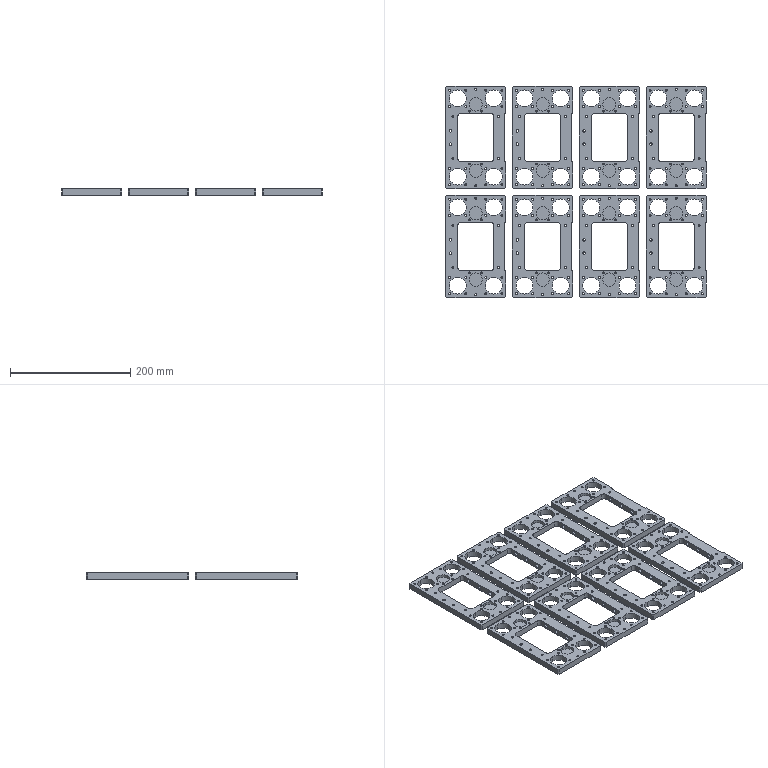NC program | NX | posted with a generic post | part box 433 x 351 x 10 mm
Lines 530 to 1335 of 15742:
(ZLEVEL_PROFILE , TOOL : D10)
N1046 T15 M6
N1048 G54
N1050 G17 G0 G90 X-221.6 Y-137.058 B0. C0. S9500 M3
N1052 G43 Z30. H15
N1054 Z1.5
N1056 G94 G1 Y-90.5 Z-0.94 F1000.
N1058 Y-7.5 F3000.
N1060 G2 X-220.106 Y-3.894 R5.1
N1062 G1 X-218.106 Y-1.894
N1064 G2 X-214.5 Y-0.4 R5.1
N1066 G1 X-118.5
N1068 G2 X-114.894 Y-1.894 R5.1
N1070 G1 X-112.894 Y-3.894
N1072 G2 X-111.4 Y-7.5 R5.1
N1074 G1 Y-50.5
N1076 G2 X-113.4 Y-54.55 R5.1
N1078 G1 Y-126.45
N1080 G2 X-111.4 Y-130.5 R5.1
N1082 G1 Y-173.5
N1084 G2 X-112.894 Y-177.106 R5.1
N1086 G1 X-114.894 Y-179.106
N1088 G2 X-118.5 Y-180.6 R5.1
N1090 G1 X-214.5
N1092 G2 X-218.106 Y-179.106 R5.1
N1094 G1 X-220.106 Y-177.106
N1096 G2 X-221.6 Y-173.5 R5.1
N1098 G1 Y-90.5
N1100 Y-7.5 Z-1.077
N1102 X-221.575 Y-7. Z-1.078
N1104 X-221.502 Y-6.505 Z-1.079
N1106 X-221.38 Y-6.02 Z-1.08
N1108 X-221.212 Y-5.548 Z-1.081
N1110 X-220.998 Y-5.096
N1112 X-220.74 Y-4.667 Z-1.082
N1114 X-220.442 Y-4.265 Z-1.083
N1116 X-220.106 Y-3.894 Z-1.084
N1118 X-218.106 Y-1.894 Z-1.089
N1120 X-217.735 Y-1.558
N1122 X-217.333 Y-1.26 Z-1.09
N1124 X-216.904 Y-1.002 Z-1.091
N1126 X-216.452 Y-0.788 Z-1.092
N1128 X-215.98 Y-0.62 Z-1.093
N1130 X-215.495 Y-0.498
N1132 X-215. Y-0.425 Z-1.094
N1134 X-214.5 Y-0.4 Z-1.095
N1136 X-118.5 Z-1.254
N1138 X-118. Y-0.425 Z-1.255
N1140 X-117.505 Y-0.498
N1142 X-117.02 Y-0.62 Z-1.256
N1144 X-116.548 Y-0.788 Z-1.257
N1146 X-116.096 Y-1.002 Z-1.258
N1148 X-115.667 Y-1.26 Z-1.259
N1150 X-115.265 Y-1.558 Z-1.26
N1152 X-114.894 Y-1.894
N1154 X-112.894 Y-3.894 Z-1.265
N1156 X-112.558 Y-4.265 Z-1.266
N1158 X-112.26 Y-4.667 Z-1.267
N1160 X-112.002 Y-5.096 Z-1.268
N1162 X-111.788 Y-5.548
N1164 X-111.62 Y-6.02 Z-1.269
N1166 X-111.498 Y-6.505 Z-1.27
N1168 X-111.425 Y-7. Z-1.271
N1170 X-111.4 Y-7.5 Z-1.272
N1172 Y-50.5 Z-1.343
N1174 X-111.421 Y-50.967 Z-1.344
N1176 X-111.486 Y-51.431
N1178 X-111.592 Y-51.886 Z-1.345
N1180 X-111.74 Y-52.33 Z-1.346
N1182 X-111.927 Y-52.758 Z-1.347
N1184 X-112.153 Y-53.168
N1186 X-112.416 Y-53.555 Z-1.348
N1188 X-112.713 Y-53.916 Z-1.349
N1190 X-113.038 Y-54.245 Z-1.35
N1192 X-113.4 Y-54.55 Z-1.351
N1194 Y-126.45 Z-1.469
N1196 X-113.034 Y-126.758 Z-1.47
N1198 X-112.713 Y-127.084 Z-1.471
N1200 X-112.416 Y-127.445 Z-1.472
N1202 X-112.153 Y-127.832 Z-1.473
N1204 X-111.927 Y-128.242
N1206 X-111.74 Y-128.67 Z-1.474
N1208 X-111.592 Y-129.114 Z-1.475
N1210 X-111.486 Y-129.569 Z-1.476
N1212 X-111.421 Y-130.033
N1214 X-111.4 Y-130.5 Z-1.477
N1216 Y-173.5 Z-1.548
N1218 X-111.425 Y-174. Z-1.549
N1220 X-111.498 Y-174.495 Z-1.55
N1222 X-111.62 Y-174.98 Z-1.551
N1224 X-111.788 Y-175.452 Z-1.552
N1226 X-112.002 Y-175.904
N1228 X-112.26 Y-176.333 Z-1.553
N1230 X-112.558 Y-176.735 Z-1.554
N1232 X-112.894 Y-177.106 Z-1.555
N1234 X-114.894 Y-179.106 Z-1.56
N1236 X-115.265 Y-179.442
N1238 X-115.667 Y-179.74 Z-1.561
N1240 X-116.096 Y-179.998 Z-1.562
N1242 X-116.548 Y-180.212 Z-1.563
N1244 X-117.02 Y-180.38 Z-1.564
N1246 X-117.505 Y-180.502 Z-1.565
N1248 X-118. Y-180.575
N1250 X-118.5 Y-180.6 Z-1.566
N1252 X-214.5 Z-1.725
N1254 X-215. Y-180.575 Z-1.726
N1256 X-215.495 Y-180.502 Z-1.727
N1258 X-215.98 Y-180.38
N1260 X-216.452 Y-180.212 Z-1.728
N1262 X-216.904 Y-179.998 Z-1.729
N1264 X-217.333 Y-179.74 Z-1.73
N1266 X-217.735 Y-179.442 Z-1.731
N1268 X-218.106 Y-179.106
N1270 X-220.106 Y-177.106 Z-1.736
N1272 X-220.442 Y-176.735 Z-1.737
N1274 X-220.74 Y-176.333 Z-1.738
N1276 X-220.998 Y-175.904 Z-1.739
N1278 X-221.212 Y-175.452
N1280 X-221.38 Y-174.98 Z-1.74
N1282 X-221.502 Y-174.495 Z-1.741
N1284 X-221.575 Y-174. Z-1.742
N1286 X-221.6 Y-173.5 Z-1.743
N1288 Y-90.5 Z-1.88
N1290 Y-7.5 Z-2.017
N1292 X-221.575 Y-7. Z-2.018
N1294 X-221.502 Y-6.505 Z-2.019
N1296 X-221.38 Y-6.02 Z-2.02
N1298 X-221.212 Y-5.548 Z-2.021
N1300 X-220.998 Y-5.096
N1302 X-220.74 Y-4.667 Z-2.022
N1304 X-220.442 Y-4.265 Z-2.023
N1306 X-220.106 Y-3.894 Z-2.024
N1308 X-218.106 Y-1.894 Z-2.029
N1310 X-217.735 Y-1.558
N1312 X-217.333 Y-1.26 Z-2.03
N1314 X-216.904 Y-1.002 Z-2.031
N1316 X-216.452 Y-0.788 Z-2.032
N1318 X-215.98 Y-0.62 Z-2.033
N1320 X-215.495 Y-0.498
N1322 X-215. Y-0.425 Z-2.034
N1324 X-214.5 Y-0.4 Z-2.035
N1326 X-118.5 Z-2.194
N1328 X-118. Y-0.425 Z-2.195
N1330 X-117.505 Y-0.498
N1332 X-117.02 Y-0.62 Z-2.196
N1334 X-116.548 Y-0.788 Z-2.197
N1336 X-116.096 Y-1.002 Z-2.198
N1338 X-115.667 Y-1.26 Z-2.199
N1340 X-115.265 Y-1.558 Z-2.2
N1342 X-114.894 Y-1.894
N1344 X-112.894 Y-3.894 Z-2.205
N1346 X-112.558 Y-4.265 Z-2.206
N1348 X-112.26 Y-4.667 Z-2.207
N1350 X-112.002 Y-5.096 Z-2.208
N1352 X-111.788 Y-5.548
N1354 X-111.62 Y-6.02 Z-2.209
N1356 X-111.498 Y-6.505 Z-2.21
N1358 X-111.425 Y-7. Z-2.211
N1360 X-111.4 Y-7.5 Z-2.212
N1362 Y-50.5 Z-2.283
N1364 X-111.421 Y-50.967 Z-2.284
N1366 X-111.486 Y-51.431
N1368 X-111.592 Y-51.886 Z-2.285
N1370 X-111.74 Y-52.33 Z-2.286
N1372 X-111.927 Y-52.758 Z-2.287
N1374 X-112.153 Y-53.168
N1376 X-112.416 Y-53.555 Z-2.288
N1378 X-112.713 Y-53.916 Z-2.289
N1380 X-113.038 Y-54.245 Z-2.29
N1382 X-113.4 Y-54.55 Z-2.291
N1384 Y-126.45 Z-2.409
N1386 X-113.034 Y-126.758 Z-2.41
N1388 X-112.713 Y-127.084 Z-2.411
N1390 X-112.416 Y-127.445 Z-2.412
N1392 X-112.153 Y-127.832 Z-2.413
N1394 X-111.927 Y-128.242
N1396 X-111.74 Y-128.67 Z-2.414
N1398 X-111.592 Y-129.114 Z-2.415
N1400 X-111.486 Y-129.569 Z-2.416
N1402 X-111.421 Y-130.033
N1404 X-111.4 Y-130.5 Z-2.417
N1406 Y-173.5 Z-2.488
N1408 X-111.425 Y-174. Z-2.489
N1410 X-111.498 Y-174.495 Z-2.49
N1412 X-111.62 Y-174.98 Z-2.491
N1414 X-111.788 Y-175.452 Z-2.492
N1416 X-112.002 Y-175.904
N1418 X-112.26 Y-176.333 Z-2.493
N1420 X-112.558 Y-176.735 Z-2.494
N1422 X-112.894 Y-177.106 Z-2.495
N1424 X-114.894 Y-179.106 Z-2.5
N1426 X-115.265 Y-179.442
N1428 X-115.667 Y-179.74 Z-2.501
N1430 X-116.096 Y-179.998 Z-2.502
N1432 X-116.548 Y-180.212 Z-2.503
N1434 X-117.02 Y-180.38 Z-2.504
N1436 X-117.505 Y-180.502 Z-2.505
N1438 X-118. Y-180.575
N1440 X-118.5 Y-180.6 Z-2.506
N1442 X-214.5 Z-2.665
N1444 X-215. Y-180.575 Z-2.666
N1446 X-215.495 Y-180.502 Z-2.667
N1448 X-215.98 Y-180.38
N1450 X-216.452 Y-180.212 Z-2.668
N1452 X-216.904 Y-179.998 Z-2.669
N1454 X-217.333 Y-179.74 Z-2.67
N1456 X-217.735 Y-179.442 Z-2.671
N1458 X-218.106 Y-179.106
N1460 X-220.106 Y-177.106 Z-2.676
N1462 X-220.442 Y-176.735 Z-2.677
N1464 X-220.74 Y-176.333 Z-2.678
N1466 X-220.998 Y-175.904 Z-2.679
N1468 X-221.212 Y-175.452
N1470 X-221.38 Y-174.98 Z-2.68
N1472 X-221.502 Y-174.495 Z-2.681
N1474 X-221.575 Y-174. Z-2.682
N1476 X-221.6 Y-173.5 Z-2.683
N1478 Y-90.5 Z-2.82
N1480 Y-7.5 Z-2.957
N1482 X-221.575 Y-7. Z-2.958
N1484 X-221.502 Y-6.505 Z-2.959
N1486 X-221.38 Y-6.02 Z-2.96
N1488 X-221.212 Y-5.548 Z-2.961
N1490 X-220.998 Y-5.096
N1492 X-220.74 Y-4.667 Z-2.962
N1494 X-220.442 Y-4.265 Z-2.963
N1496 X-220.106 Y-3.894 Z-2.964
N1498 X-218.106 Y-1.894 Z-2.969
N1500 X-217.735 Y-1.558
N1502 X-217.333 Y-1.26 Z-2.97
N1504 X-216.904 Y-1.002 Z-2.971
N1506 X-216.452 Y-0.788 Z-2.972
N1508 X-215.98 Y-0.62 Z-2.973
N1510 X-215.495 Y-0.498
N1512 X-215. Y-0.425 Z-2.974
N1514 X-214.5 Y-0.4 Z-2.975
N1516 X-118.5 Z-3.134
N1518 X-118. Y-0.425 Z-3.135
N1520 X-117.505 Y-0.498
N1522 X-117.02 Y-0.62 Z-3.136
N1524 X-116.548 Y-0.788 Z-3.137
N1526 X-116.096 Y-1.002 Z-3.138
N1528 X-115.667 Y-1.26 Z-3.139
N1530 X-115.265 Y-1.558 Z-3.14
N1532 X-114.894 Y-1.894
N1534 X-112.894 Y-3.894 Z-3.145
N1536 X-112.558 Y-4.265 Z-3.146
N1538 X-112.26 Y-4.667 Z-3.147
N1540 X-112.002 Y-5.096 Z-3.148
N1542 X-111.788 Y-5.548
N1544 X-111.62 Y-6.02 Z-3.149
N1546 X-111.498 Y-6.505 Z-3.15
N1548 X-111.425 Y-7. Z-3.151
N1550 X-111.4 Y-7.5 Z-3.152
N1552 Y-50.5 Z-3.223
N1554 X-111.421 Y-50.967 Z-3.224
N1556 X-111.486 Y-51.431
N1558 X-111.592 Y-51.886 Z-3.225
N1560 X-111.74 Y-52.33 Z-3.226
N1562 X-111.927 Y-52.758 Z-3.227
N1564 X-112.153 Y-53.168
N1566 X-112.416 Y-53.555 Z-3.228
N1568 X-112.713 Y-53.916 Z-3.229
N1570 X-113.038 Y-54.245 Z-3.23
N1572 X-113.4 Y-54.55 Z-3.231
N1574 Y-126.45 Z-3.349
N1576 X-113.034 Y-126.758 Z-3.35
N1578 X-112.713 Y-127.084 Z-3.351
N1580 X-112.416 Y-127.445 Z-3.352
N1582 X-112.153 Y-127.832 Z-3.353
N1584 X-111.927 Y-128.242
N1586 X-111.74 Y-128.67 Z-3.354
N1588 X-111.592 Y-129.114 Z-3.355
N1590 X-111.486 Y-129.569 Z-3.356
N1592 X-111.421 Y-130.033
N1594 X-111.4 Y-130.5 Z-3.357
N1596 Y-173.5 Z-3.428
N1598 X-111.425 Y-174. Z-3.429
N1600 X-111.498 Y-174.495 Z-3.43
N1602 X-111.62 Y-174.98 Z-3.431
N1604 X-111.788 Y-175.452 Z-3.432
N1606 X-112.002 Y-175.904
N1608 X-112.26 Y-176.333 Z-3.433
N1610 X-112.558 Y-176.735 Z-3.434
N1612 X-112.894 Y-177.106 Z-3.435
N1614 X-114.894 Y-179.106 Z-3.44
N1616 X-115.265 Y-179.442
N1618 X-115.667 Y-179.74 Z-3.441
N1620 X-116.096 Y-179.998 Z-3.442
N1622 X-116.548 Y-180.212 Z-3.443
N1624 X-117.02 Y-180.38 Z-3.444
N1626 X-117.505 Y-180.502 Z-3.445
N1628 X-118. Y-180.575
N1630 X-118.5 Y-180.6 Z-3.446
N1632 X-214.5 Z-3.605
N1634 X-215. Y-180.575 Z-3.606
N1636 X-215.495 Y-180.502 Z-3.607
N1638 X-215.98 Y-180.38
N1640 X-216.452 Y-180.212 Z-3.608
N1642 X-216.904 Y-179.998 Z-3.609
N1644 X-217.333 Y-179.74 Z-3.61
N1646 X-217.735 Y-179.442 Z-3.611
N1648 X-218.106 Y-179.106
N1650 X-220.106 Y-177.106 Z-3.616
N1652 X-220.442 Y-176.735 Z-3.617
N1654 X-220.74 Y-176.333 Z-3.618
N1656 X-220.998 Y-175.904 Z-3.619
N1658 X-221.212 Y-175.452
N1660 X-221.38 Y-174.98 Z-3.62
N1662 X-221.502 Y-174.495 Z-3.621
N1664 X-221.575 Y-174. Z-3.622
N1666 X-221.6 Y-173.5 Z-3.623
N1668 Y-90.5 Z-3.76
N1670 Y-7.5 Z-3.897
N1672 X-221.575 Y-7. Z-3.898
N1674 X-221.502 Y-6.505 Z-3.899
N1676 X-221.38 Y-6.02 Z-3.9
N1678 X-221.212 Y-5.548 Z-3.901
N1680 X-220.998 Y-5.096
N1682 X-220.74 Y-4.667 Z-3.902
N1684 X-220.442 Y-4.265 Z-3.903
N1686 X-220.106 Y-3.894 Z-3.904
N1688 X-218.106 Y-1.894 Z-3.909
N1690 X-217.735 Y-1.558
N1692 X-217.333 Y-1.26 Z-3.91
N1694 X-216.904 Y-1.002 Z-3.911
N1696 X-216.452 Y-0.788 Z-3.912
N1698 X-215.98 Y-0.62 Z-3.913
N1700 X-215.495 Y-0.498
N1702 X-215. Y-0.425 Z-3.914
N1704 X-214.5 Y-0.4 Z-3.915
N1706 X-118.5 Z-4.074
N1708 X-118. Y-0.425 Z-4.075
N1710 X-117.505 Y-0.498
N1712 X-117.02 Y-0.62 Z-4.076
N1714 X-116.548 Y-0.788 Z-4.077
N1716 X-116.096 Y-1.002 Z-4.078
N1718 X-115.667 Y-1.26 Z-4.079
N1720 X-115.265 Y-1.558 Z-4.08
N1722 X-114.894 Y-1.894
N1724 X-112.894 Y-3.894 Z-4.085
N1726 X-112.558 Y-4.265 Z-4.086
N1728 X-112.26 Y-4.667 Z-4.087
N1730 X-112.002 Y-5.096 Z-4.088
N1732 X-111.788 Y-5.548
N1734 X-111.62 Y-6.02 Z-4.089
N1736 X-111.498 Y-6.505 Z-4.09
N1738 X-111.425 Y-7. Z-4.091
N1740 X-111.4 Y-7.5 Z-4.092
N1742 Y-50.5 Z-4.163
N1744 X-111.421 Y-50.967 Z-4.164
N1746 X-111.486 Y-51.431
N1748 X-111.592 Y-51.886 Z-4.165
N1750 X-111.74 Y-52.33 Z-4.166
N1752 X-111.927 Y-52.758 Z-4.167
N1754 X-112.153 Y-53.168
N1756 X-112.416 Y-53.555 Z-4.168
N1758 X-112.713 Y-53.916 Z-4.169
N1760 X-113.038 Y-54.245 Z-4.17
N1762 X-113.4 Y-54.55 Z-4.171
N1764 Y-126.45 Z-4.289
N1766 X-113.034 Y-126.758 Z-4.29
N1768 X-112.713 Y-127.084 Z-4.291
N1770 X-112.416 Y-127.445 Z-4.292
N1772 X-112.153 Y-127.832 Z-4.293
N1774 X-111.927 Y-128.242
N1776 X-111.74 Y-128.67 Z-4.294
N1778 X-111.592 Y-129.114 Z-4.295
N1780 X-111.486 Y-129.569 Z-4.296
N1782 X-111.421 Y-130.033
N1784 X-111.4 Y-130.5 Z-4.297
N1786 Y-173.5 Z-4.368
N1788 X-111.425 Y-174. Z-4.369
N1790 X-111.498 Y-174.495 Z-4.37
N1792 X-111.62 Y-174.98 Z-4.371
N1794 X-111.788 Y-175.452 Z-4.372
N1796 X-112.002 Y-175.904
N1798 X-112.26 Y-176.333 Z-4.373
N1800 X-112.558 Y-176.735 Z-4.374
N1802 X-112.894 Y-177.106 Z-4.375
N1804 X-114.894 Y-179.106 Z-4.38
N1806 X-115.265 Y-179.442
N1808 X-115.667 Y-179.74 Z-4.381
N1810 X-116.096 Y-179.998 Z-4.382
N1812 X-116.548 Y-180.212 Z-4.383
N1814 X-117.02 Y-180.38 Z-4.384
N1816 X-117.505 Y-180.502 Z-4.385
N1818 X-118. Y-180.575
N1820 X-118.5 Y-180.6 Z-4.386
N1822 X-214.5 Z-4.545
N1824 X-215. Y-180.575 Z-4.546
N1826 X-215.495 Y-180.502 Z-4.547
N1828 X-215.98 Y-180.38
N1830 X-216.452 Y-180.212 Z-4.548
N1832 X-216.904 Y-179.998 Z-4.549
N1834 X-217.333 Y-179.74 Z-4.55
N1836 X-217.735 Y-179.442 Z-4.551
N1838 X-218.106 Y-179.106
N1840 X-220.106 Y-177.106 Z-4.556
N1842 X-220.442 Y-176.735 Z-4.557
N1844 X-220.74 Y-176.333 Z-4.558
N1846 X-220.998 Y-175.904 Z-4.559
N1848 X-221.212 Y-175.452
N1850 X-221.38 Y-174.98 Z-4.56
N1852 X-221.502 Y-174.495 Z-4.561
N1854 X-221.575 Y-174. Z-4.562
N1856 X-221.6 Y-173.5 Z-4.563
N1858 Y-90.5 Z-4.7
N1860 Y-7.5 Z-4.837
N1862 X-221.575 Y-7. Z-4.838
N1864 X-221.502 Y-6.505 Z-4.839
N1866 X-221.38 Y-6.02 Z-4.84
N1868 X-221.212 Y-5.548 Z-4.841
N1870 X-220.998 Y-5.096
N1872 X-220.74 Y-4.667 Z-4.842
N1874 X-220.442 Y-4.265 Z-4.843
N1876 X-220.106 Y-3.894 Z-4.844
N1878 X-218.106 Y-1.894 Z-4.849
N1880 X-217.735 Y-1.558
N1882 X-217.333 Y-1.26 Z-4.85
N1884 X-216.904 Y-1.002 Z-4.851
N1886 X-216.452 Y-0.788 Z-4.852
N1888 X-215.98 Y-0.62 Z-4.853
N1890 X-215.495 Y-0.498
N1892 X-215. Y-0.425 Z-4.854
N1894 X-214.5 Y-0.4 Z-4.855
N1896 X-118.5 Z-5.014
N1898 X-118. Y-0.425 Z-5.015
N1900 X-117.505 Y-0.498
N1902 X-117.02 Y-0.62 Z-5.016
N1904 X-116.548 Y-0.788 Z-5.017
N1906 X-116.096 Y-1.002 Z-5.018
N1908 X-115.667 Y-1.26 Z-5.019
N1910 X-115.265 Y-1.558 Z-5.02
N1912 X-114.894 Y-1.894
N1914 X-112.894 Y-3.894 Z-5.025
N1916 X-112.558 Y-4.265 Z-5.026
N1918 X-112.26 Y-4.667 Z-5.027
N1920 X-112.002 Y-5.096 Z-5.028
N1922 X-111.788 Y-5.548
N1924 X-111.62 Y-6.02 Z-5.029
N1926 X-111.498 Y-6.505 Z-5.03
N1928 X-111.425 Y-7. Z-5.031
N1930 X-111.4 Y-7.5 Z-5.032
N1932 Y-50.5 Z-5.103
N1934 X-111.421 Y-50.967 Z-5.104
N1936 X-111.486 Y-51.431
N1938 X-111.592 Y-51.886 Z-5.105
N1940 X-111.74 Y-52.33 Z-5.106
N1942 X-111.927 Y-52.758 Z-5.107
N1944 X-112.153 Y-53.168
N1946 X-112.416 Y-53.555 Z-5.108
N1948 X-112.713 Y-53.916 Z-5.109
N1950 X-113.038 Y-54.245 Z-5.11
N1952 X-113.4 Y-54.55 Z-5.111
N1954 Y-126.45 Z-5.229
N1956 X-113.034 Y-126.758 Z-5.23
N1958 X-112.713 Y-127.084 Z-5.231
N1960 X-112.416 Y-127.445 Z-5.232
N1962 X-112.153 Y-127.832 Z-5.233
N1964 X-111.927 Y-128.242
N1966 X-111.74 Y-128.67 Z-5.234
N1968 X-111.592 Y-129.114 Z-5.235
N1970 X-111.486 Y-129.569 Z-5.236
N1972 X-111.421 Y-130.033
N1974 X-111.4 Y-130.5 Z-5.237
N1976 Y-173.5 Z-5.308
N1978 X-111.425 Y-174. Z-5.309
N1980 X-111.498 Y-174.495 Z-5.31
N1982 X-111.62 Y-174.98 Z-5.311
N1984 X-111.788 Y-175.452 Z-5.312
N1986 X-112.002 Y-175.904
N1988 X-112.26 Y-176.333 Z-5.313
N1990 X-112.558 Y-176.735 Z-5.314
N1992 X-112.894 Y-177.106 Z-5.315
N1994 X-114.894 Y-179.106 Z-5.32
N1996 X-115.265 Y-179.442
N1998 X-115.667 Y-179.74 Z-5.321
N2000 X-116.096 Y-179.998 Z-5.322
N2002 X-116.548 Y-180.212 Z-5.323
N2004 X-117.02 Y-180.38 Z-5.324
N2006 X-117.505 Y-180.502 Z-5.325
N2008 X-118. Y-180.575
N2010 X-118.5 Y-180.6 Z-5.326
N2012 X-214.5 Z-5.485
N2014 X-215. Y-180.575 Z-5.486
N2016 X-215.495 Y-180.502 Z-5.487
N2018 X-215.98 Y-180.38
N2020 X-216.452 Y-180.212 Z-5.488
N2022 X-216.904 Y-179.998 Z-5.489
N2024 X-217.333 Y-179.74 Z-5.49
N2026 X-217.735 Y-179.442 Z-5.491
N2028 X-218.106 Y-179.106
N2030 X-220.106 Y-177.106 Z-5.496
N2032 X-220.442 Y-176.735 Z-5.497
N2034 X-220.74 Y-176.333 Z-5.498
N2036 X-220.998 Y-175.904 Z-5.499
N2038 X-221.212 Y-175.452
N2040 X-221.38 Y-174.98 Z-5.5
N2042 X-221.502 Y-174.495 Z-5.501
N2044 X-221.575 Y-174. Z-5.502
N2046 X-221.6 Y-173.5 Z-5.503
N2048 Y-90.5 Z-5.64
N2050 Y-7.5 Z-5.777
N2052 X-221.575 Y-7. Z-5.778
N2054 X-221.502 Y-6.505 Z-5.779
N2056 X-221.38 Y-6.02 Z-5.78
N2058 X-221.212 Y-5.548 Z-5.781
N2060 X-220.998 Y-5.096
N2062 X-220.74 Y-4.667 Z-5.782
N2064 X-220.442 Y-4.265 Z-5.783
N2066 X-220.106 Y-3.894 Z-5.784
N2068 X-218.106 Y-1.894 Z-5.789
N2070 X-217.735 Y-1.558
N2072 X-217.333 Y-1.26 Z-5.79
N2074 X-216.904 Y-1.002 Z-5.791
N2076 X-216.452 Y-0.788 Z-5.792
N2078 X-215.98 Y-0.62 Z-5.793
N2080 X-215.495 Y-0.498
N2082 X-215. Y-0.425 Z-5.794
N2084 X-214.5 Y-0.4 Z-5.795
N2086 X-118.5 Z-5.954
N2088 X-118. Y-0.425 Z-5.955
N2090 X-117.505 Y-0.498
N2092 X-117.02 Y-0.62 Z-5.956
N2094 X-116.548 Y-0.788 Z-5.957
N2096 X-116.096 Y-1.002 Z-5.958
N2098 X-115.667 Y-1.26 Z-5.959
N2100 X-115.265 Y-1.558 Z-5.96
N2102 X-114.894 Y-1.894
N2104 X-112.894 Y-3.894 Z-5.965
N2106 X-112.558 Y-4.265 Z-5.966
N2108 X-112.26 Y-4.667 Z-5.967
N2110 X-112.002 Y-5.096 Z-5.968
N2112 X-111.788 Y-5.548
N2114 X-111.62 Y-6.02 Z-5.969
N2116 X-111.498 Y-6.505 Z-5.97
N2118 X-111.425 Y-7. Z-5.971
N2120 X-111.4 Y-7.5 Z-5.972
N2122 Y-50.5 Z-6.043
N2124 X-111.421 Y-50.967 Z-6.044
N2126 X-111.486 Y-51.431
N2128 X-111.592 Y-51.886 Z-6.045
N2130 X-111.74 Y-52.33 Z-6.046
N2132 X-111.927 Y-52.758 Z-6.047
N2134 X-112.153 Y-53.168
N2136 X-112.416 Y-53.555 Z-6.048
N2138 X-112.713 Y-53.916 Z-6.049
N2140 X-113.038 Y-54.245 Z-6.05
N2142 X-113.4 Y-54.55 Z-6.051
N2144 Y-126.45 Z-6.169
N2146 X-113.034 Y-126.758 Z-6.17
N2148 X-112.713 Y-127.084 Z-6.171
N2150 X-112.416 Y-127.445 Z-6.172
N2152 X-112.153 Y-127.832 Z-6.173
N2154 X-111.927 Y-128.242
N2156 X-111.74 Y-128.67 Z-6.174
N2158 X-111.592 Y-129.114 Z-6.175
N2160 X-111.486 Y-129.569 Z-6.176
N2162 X-111.421 Y-130.033
N2164 X-111.4 Y-130.5 Z-6.177
N2166 Y-173.5 Z-6.248
N2168 X-111.425 Y-174. Z-6.249
N2170 X-111.498 Y-174.495 Z-6.25
N2172 X-111.62 Y-174.98 Z-6.251
N2174 X-111.788 Y-175.452 Z-6.252
N2176 X-112.002 Y-175.904
N2178 X-112.26 Y-176.333 Z-6.253
N2180 X-112.558 Y-176.735 Z-6.254
N2182 X-112.894 Y-177.106 Z-6.255
N2184 X-114.894 Y-179.106 Z-6.26
N2186 X-115.265 Y-179.442
N2188 X-115.667 Y-179.74 Z-6.261
N2190 X-116.096 Y-179.998 Z-6.262
N2192 X-116.548 Y-180.212 Z-6.263
N2194 X-117.02 Y-180.38 Z-6.264
N2196 X-117.505 Y-180.502 Z-6.265
N2198 X-118. Y-180.575
N2200 X-118.5 Y-180.6 Z-6.266
N2202 X-214.5 Z-6.425
N2204 X-215. Y-180.575 Z-6.426
N2206 X-215.495 Y-180.502 Z-6.427
N2208 X-215.98 Y-180.38
N2210 X-216.452 Y-180.212 Z-6.428
N2212 X-216.904 Y-179.998 Z-6.429
N2214 X-217.333 Y-179.74 Z-6.43
N2216 X-217.735 Y-179.442 Z-6.431
N2218 X-218.106 Y-179.106
N2220 X-220.106 Y-177.106 Z-6.436
N2222 X-220.442 Y-176.735 Z-6.437
N2224 X-220.74 Y-176.333 Z-6.438
N2226 X-220.998 Y-175.904 Z-6.439
N2228 X-221.212 Y-175.452
N2230 X-221.38 Y-174.98 Z-6.44
N2232 X-221.502 Y-174.495 Z-6.441
N2234 X-221.575 Y-174. Z-6.442
N2236 X-221.6 Y-173.5 Z-6.443
N2238 Y-90.5 Z-6.58
N2240 Y-7.5 Z-6.717
N2242 X-221.575 Y-7. Z-6.718
N2244 X-221.502 Y-6.505 Z-6.719
N2246 X-221.38 Y-6.02 Z-6.72
N2248 X-221.212 Y-5.548 Z-6.721
N2250 X-220.998 Y-5.096
N2252 X-220.74 Y-4.667 Z-6.722
N2254 X-220.442 Y-4.265 Z-6.723
N2256 X-220.106 Y-3.894 Z-6.724
N2258 X-218.106 Y-1.894 Z-6.729
N2260 X-217.735 Y-1.558
N2262 X-217.333 Y-1.26 Z-6.73
N2264 X-216.904 Y-1.002 Z-6.731
N2266 X-216.452 Y-0.788 Z-6.732
N2268 X-215.98 Y-0.62 Z-6.733
N2270 X-215.495 Y-0.498
N2272 X-215. Y-0.425 Z-6.734
N2274 X-214.5 Y-0.4 Z-6.735
N2276 X-118.5 Z-6.894
N2278 X-118. Y-0.425 Z-6.895
N2280 X-117.505 Y-0.498
N2282 X-117.02 Y-0.62 Z-6.896
N2284 X-116.548 Y-0.788 Z-6.897
N2286 X-116.096 Y-1.002 Z-6.898
N2288 X-115.667 Y-1.26 Z-6.899
N2290 X-115.265 Y-1.558 Z-6.9
N2292 X-114.894 Y-1.894
N2294 X-112.894 Y-3.894 Z-6.905
N2296 X-112.558 Y-4.265 Z-6.906
N2298 X-112.26 Y-4.667 Z-6.907
N2300 X-112.002 Y-5.096 Z-6.908
N2302 X-111.788 Y-5.548
N2304 X-111.62 Y-6.02 Z-6.909
N2306 X-111.498 Y-6.505 Z-6.91
N2308 X-111.425 Y-7. Z-6.911
N2310 X-111.4 Y-7.5 Z-6.912
N2312 Y-50.5 Z-6.983
N2314 X-111.421 Y-50.967 Z-6.984
N2316 X-111.486 Y-51.431
N2318 X-111.592 Y-51.886 Z-6.985
N2320 X-111.74 Y-52.33 Z-6.986
N2322 X-111.927 Y-52.758 Z-6.987
N2324 X-112.153 Y-53.168
N2326 X-112.416 Y-53.555 Z-6.988
N2328 X-112.713 Y-53.916 Z-6.989
N2330 X-113.038 Y-54.245 Z-6.99
N2332 X-113.4 Y-54.55 Z-6.991
N2334 Y-126.45 Z-7.109
N2336 X-113.034 Y-126.758 Z-7.11
N2338 X-112.713 Y-127.084 Z-7.111
N2340 X-112.416 Y-127.445 Z-7.112
N2342 X-112.153 Y-127.832 Z-7.113
N2344 X-111.927 Y-128.242
N2346 X-111.74 Y-128.67 Z-7.114
N2348 X-111.592 Y-129.114 Z-7.115
N2350 X-111.486 Y-129.569 Z-7.116
N2352 X-111.421 Y-130.033
N2354 X-111.4 Y-130.5 Z-7.117
N2356 Y-173.5 Z-7.188
N2358 X-111.425 Y-174. Z-7.189
N2360 X-111.498 Y-174.495 Z-7.19
N2362 X-111.62 Y-174.98 Z-7.191
N2364 X-111.788 Y-175.452 Z-7.192
N2366 X-112.002 Y-175.904
N2368 X-112.26 Y-176.333 Z-7.193
N2370 X-112.558 Y-176.735 Z-7.194
N2372 X-112.894 Y-177.106 Z-7.195
N2374 X-114.894 Y-179.106 Z-7.2
N2376 X-115.265 Y-179.442
N2378 X-115.667 Y-179.74 Z-7.201
N2380 X-116.096 Y-179.998 Z-7.202
N2382 X-116.548 Y-180.212 Z-7.203
N2384 X-117.02 Y-180.38 Z-7.204
N2386 X-117.505 Y-180.502 Z-7.205
N2388 X-118. Y-180.575
N2390 X-118.5 Y-180.6 Z-7.206
N2392 X-214.5 Z-7.365
N2394 X-215. Y-180.575 Z-7.366
N2396 X-215.495 Y-180.502 Z-7.367
N2398 X-215.98 Y-180.38
N2400 X-216.452 Y-180.212 Z-7.368
N2402 X-216.904 Y-179.998 Z-7.369
N2404 X-217.333 Y-179.74 Z-7.37
N2406 X-217.735 Y-179.442 Z-7.371
N2408 X-218.106 Y-179.106
N2410 X-220.106 Y-177.106 Z-7.376
N2412 X-220.442 Y-176.735 Z-7.377
N2414 X-220.74 Y-176.333 Z-7.378
N2416 X-220.998 Y-175.904 Z-7.379
N2418 X-221.212 Y-175.452
N2420 X-221.38 Y-174.98 Z-7.38
N2422 X-221.502 Y-174.495 Z-7.381
N2424 X-221.575 Y-174. Z-7.382
N2426 X-221.6 Y-173.5 Z-7.383
N2428 Y-90.5 Z-7.52
N2430 Y-7.5 Z-7.657
N2432 X-221.575 Y-7. Z-7.658
N2434 X-221.502 Y-6.505 Z-7.659
N2436 X-221.38 Y-6.02 Z-7.66
N2438 X-221.212 Y-5.548 Z-7.661
N2440 X-220.998 Y-5.096
N2442 X-220.74 Y-4.667 Z-7.662
N2444 X-220.442 Y-4.265 Z-7.663
N2446 X-220.106 Y-3.894 Z-7.664
N2448 X-218.106 Y-1.894 Z-7.669
N2450 X-217.735 Y-1.558
N2452 X-217.333 Y-1.26 Z-7.67
N2454 X-216.904 Y-1.002 Z-7.671
N2456 X-216.452 Y-0.788 Z-7.672
N2458 X-215.98 Y-0.62 Z-7.673
N2460 X-215.495 Y-0.498
N2462 X-215. Y-0.425 Z-7.674
N2464 X-214.5 Y-0.4 Z-7.675
N2466 X-118.5 Z-7.834
N2468 X-118. Y-0.425 Z-7.835
N2470 X-117.505 Y-0.498
N2472 X-117.02 Y-0.62 Z-7.836
N2474 X-116.548 Y-0.788 Z-7.837
N2476 X-116.096 Y-1.002 Z-7.838
N2478 X-115.667 Y-1.26 Z-7.839
N2480 X-115.265 Y-1.558 Z-7.84
N2482 X-114.894 Y-1.894
N2484 X-112.894 Y-3.894 Z-7.845
N2486 X-112.558 Y-4.265 Z-7.846
N2488 X-112.26 Y-4.667 Z-7.847
N2490 X-112.002 Y-5.096 Z-7.848
N2492 X-111.788 Y-5.548
N2494 X-111.62 Y-6.02 Z-7.849
N2496 X-111.498 Y-6.505 Z-7.85
N2498 X-111.425 Y-7. Z-7.851
N2500 X-111.4 Y-7.5 Z-7.852
N2502 Y-50.5 Z-7.923
N2504 X-111.421 Y-50.967 Z-7.924
N2506 X-111.486 Y-51.431
N2508 X-111.592 Y-51.886 Z-7.925
N2510 X-111.74 Y-52.33 Z-7.926
N2512 X-111.927 Y-52.758 Z-7.927
N2514 X-112.153 Y-53.168
N2516 X-112.416 Y-53.555 Z-7.928
N2518 X-112.713 Y-53.916 Z-7.929
N2520 X-113.038 Y-54.245 Z-7.93
N2522 X-113.4 Y-54.55 Z-7.931
N2524 Y-126.45 Z-8.049
N2526 X-113.034 Y-126.758 Z-8.05
N2528 X-112.713 Y-127.084 Z-8.051
N2530 X-112.416 Y-127.445 Z-8.052
N2532 X-112.153 Y-127.832 Z-8.053
N2534 X-111.927 Y-128.242
N2536 X-111.74 Y-128.67 Z-8.054
N2538 X-111.592 Y-129.114 Z-8.055
N2540 X-111.486 Y-129.569 Z-8.056
N2542 X-111.421 Y-130.033
N2544 X-111.4 Y-130.5 Z-8.057
N2546 Y-173.5 Z-8.128
N2548 X-111.425 Y-174. Z-8.129
N2550 X-111.498 Y-174.495 Z-8.13
N2552 X-111.62 Y-174.98 Z-8.131
N2554 X-111.788 Y-175.452 Z-8.132
N2556 X-112.002 Y-175.904
N2558 X-112.26 Y-176.333 Z-8.133
N2560 X-112.558 Y-176.735 Z-8.134
N2562 X-112.894 Y-177.106 Z-8.135
N2564 X-114.894 Y-179.106 Z-8.14
N2566 X-115.265 Y-179.442
N2568 X-115.667 Y-179.74 Z-8.141
N2570 X-116.096 Y-179.998 Z-8.142
N2572 X-116.548 Y-180.212 Z-8.143
N2574 X-117.02 Y-180.38 Z-8.144
N2576 X-117.505 Y-180.502 Z-8.145
N2578 X-118. Y-180.575
N2580 X-118.5 Y-180.6 Z-8.146
N2582 X-214.5 Z-8.305
N2584 X-215. Y-180.575 Z-8.306
N2586 X-215.495 Y-180.502 Z-8.307
N2588 X-215.98 Y-180.38
N2590 X-216.452 Y-180.212 Z-8.308
N2592 X-216.904 Y-179.998 Z-8.309
N2594 X-217.333 Y-179.74 Z-8.31
N2596 X-217.735 Y-179.442 Z-8.311
N2598 X-218.106 Y-179.106
N2600 X-220.106 Y-177.106 Z-8.316
N2602 X-220.442 Y-176.735 Z-8.317
N2604 X-220.74 Y-176.333 Z-8.318
N2606 X-220.998 Y-175.904 Z-8.319
N2608 X-221.212 Y-175.452
N2610 X-221.38 Y-174.98 Z-8.32
N2612 X-221.502 Y-174.495 Z-8.321
N2614 X-221.575 Y-174. Z-8.322
N2616 X-221.6 Y-173.5 Z-8.323
N2618 Y-90.5 Z-8.46
N2620 Y-7.5 Z-8.597
N2622 X-221.575 Y-7. Z-8.598
N2624 X-221.502 Y-6.505 Z-8.599
N2626 X-221.38 Y-6.02 Z-8.6
N2628 X-221.212 Y-5.548 Z-8.601
N2630 X-220.998 Y-5.096
N2632 X-220.74 Y-4.667 Z-8.602
N2634 X-220.442 Y-4.265 Z-8.603
N2636 X-220.106 Y-3.894 Z-8.604
N2638 X-218.106 Y-1.894 Z-8.609
N2640 X-217.735 Y-1.558
N2642 X-217.333 Y-1.26 Z-8.61
N2644 X-216.904 Y-1.002 Z-8.611
N2646 X-216.452 Y-0.788 Z-8.612
N2648 X-215.98 Y-0.62 Z-8.613
N2650 X-215.495 Y-0.498